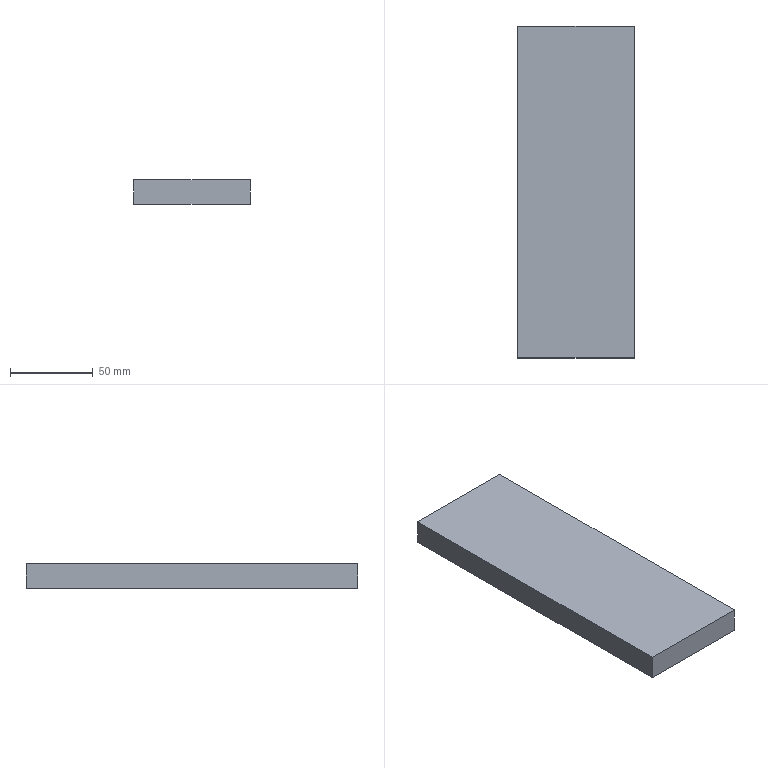Part | SolidWorks | features Extrusion 1 | 1 solid | 6 faces | box 70 x 200 x 15 mm | volume 210000 mm3 | plane 6
STEP:
#1=CARTESIAN_POINT('',(-35.,100.,-7.5));
#2=VERTEX_POINT('',#1);
#3=CARTESIAN_POINT('',(-35.,-100.,-7.5));
#4=VERTEX_POINT('',#3);
#5=CARTESIAN_POINT('',(-35.,-100.,-7.5));
#6=DIRECTION('',(0.,-1.,0.));
#7=VECTOR('',#6,1000.);
#8=LINE('',#5,#7);
#9=EDGE_CURVE('',#2,#4,#8,.T.);
#10=ORIENTED_EDGE('',*,*,#9,.T.);
#11=CARTESIAN_POINT('',(-35.,-100.,7.5));
#12=VERTEX_POINT('',#11);
#13=CARTESIAN_POINT('',(-35.,-100.,7.5));
#14=DIRECTION('',(0.,0.,-1.));
#15=VECTOR('',#14,1000.);
#16=LINE('',#13,#15);
#17=EDGE_CURVE('',#12,#4,#16,.T.);
#18=ORIENTED_EDGE('',*,*,#17,.F.);
#19=CARTESIAN_POINT('',(-35.,100.,7.5));
#20=VERTEX_POINT('',#19);
#21=CARTESIAN_POINT('',(-35.,-100.,7.5));
#22=DIRECTION('',(0.,-1.,0.));
#23=VECTOR('',#22,1000.);
#24=LINE('',#21,#23);
#25=EDGE_CURVE('',#20,#12,#24,.T.);
#26=ORIENTED_EDGE('',*,*,#25,.F.);
#27=CARTESIAN_POINT('',(-35.,100.,7.5));
#28=DIRECTION('',(0.,0.,-1.));
#29=VECTOR('',#28,1000.);
#30=LINE('',#27,#29);
#31=EDGE_CURVE('',#20,#2,#30,.T.);
#32=ORIENTED_EDGE('',*,*,#31,.T.);
#33=EDGE_LOOP('',(#10,#18,#26,#32));
#34=FACE_OUTER_BOUND('',#33,.T.);
#35=CARTESIAN_POINT('',(-35.,-100.,7.5));
#36=DIRECTION('',(1.,0.,0.));
#37=DIRECTION('',(0.,0.,-1.));
#38=AXIS2_PLACEMENT_3D('',#35,#36,#37);
#39=PLANE('',#38);
#40=ADVANCED_FACE('',(#34),#39,.F.);
#41=CARTESIAN_POINT('',(35.,-100.,-7.5));
#42=VERTEX_POINT('',#41);
#43=CARTESIAN_POINT('',(35.,-100.,-7.5));
#44=DIRECTION('',(1.,0.,0.));
#45=VECTOR('',#44,1000.);
#46=LINE('',#43,#45);
#47=EDGE_CURVE('',#4,#42,#46,.T.);
#48=ORIENTED_EDGE('',*,*,#47,.T.);
#49=CARTESIAN_POINT('',(35.,-100.,7.5));
#50=VERTEX_POINT('',#49);
#51=CARTESIAN_POINT('',(35.,-100.,7.5));
#52=DIRECTION('',(0.,0.,-1.));
#53=VECTOR('',#52,1000.);
#54=LINE('',#51,#53);
#55=EDGE_CURVE('',#50,#42,#54,.T.);
#56=ORIENTED_EDGE('',*,*,#55,.F.);
#57=CARTESIAN_POINT('',(35.,-100.,7.5));
#58=DIRECTION('',(1.,0.,0.));
#59=VECTOR('',#58,1000.);
#60=LINE('',#57,#59);
#61=EDGE_CURVE('',#12,#50,#60,.T.);
#62=ORIENTED_EDGE('',*,*,#61,.F.);
#63=ORIENTED_EDGE('',*,*,#17,.T.);
#64=EDGE_LOOP('',(#48,#56,#62,#63));
#65=FACE_OUTER_BOUND('',#64,.T.);
#66=CARTESIAN_POINT('',(35.,-100.,7.5));
#67=DIRECTION('',(0.,1.,0.));
#68=DIRECTION('',(0.,0.,1.));
#69=AXIS2_PLACEMENT_3D('',#66,#67,#68);
#70=PLANE('',#69);
#71=ADVANCED_FACE('',(#65),#70,.F.);
#72=CARTESIAN_POINT('',(35.,100.,-7.5));
#73=VERTEX_POINT('',#72);
#74=CARTESIAN_POINT('',(35.,-100.,-7.5));
#75=DIRECTION('',(0.,1.,0.));
#76=VECTOR('',#75,1000.);
#77=LINE('',#74,#76);
#78=EDGE_CURVE('',#42,#73,#77,.T.);
#79=ORIENTED_EDGE('',*,*,#78,.T.);
#80=CARTESIAN_POINT('',(35.,100.,7.5));
#81=VERTEX_POINT('',#80);
#82=CARTESIAN_POINT('',(35.,100.,7.5));
#83=DIRECTION('',(0.,0.,-1.));
#84=VECTOR('',#83,1000.);
#85=LINE('',#82,#84);
#86=EDGE_CURVE('',#81,#73,#85,.T.);
#87=ORIENTED_EDGE('',*,*,#86,.F.);
#88=CARTESIAN_POINT('',(35.,-100.,7.5));
#89=DIRECTION('',(0.,1.,0.));
#90=VECTOR('',#89,1000.);
#91=LINE('',#88,#90);
#92=EDGE_CURVE('',#50,#81,#91,.T.);
#93=ORIENTED_EDGE('',*,*,#92,.F.);
#94=ORIENTED_EDGE('',*,*,#55,.T.);
#95=EDGE_LOOP('',(#79,#87,#93,#94));
#96=FACE_OUTER_BOUND('',#95,.T.);
#97=CARTESIAN_POINT('',(35.,-100.,7.5));
#98=DIRECTION('',(-1.,0.,0.));
#99=DIRECTION('',(0.,0.,1.));
#100=AXIS2_PLACEMENT_3D('',#97,#98,#99);
#101=PLANE('',#100);
#102=ADVANCED_FACE('',(#96),#101,.F.);
#103=CARTESIAN_POINT('',(35.,100.,-7.5));
#104=DIRECTION('',(-1.,0.,0.));
#105=VECTOR('',#104,1000.);
#106=LINE('',#103,#105);
#107=EDGE_CURVE('',#73,#2,#106,.T.);
#108=ORIENTED_EDGE('',*,*,#107,.T.);
#109=ORIENTED_EDGE('',*,*,#31,.F.);
#110=CARTESIAN_POINT('',(35.,100.,7.5));
#111=DIRECTION('',(-1.,0.,0.));
#112=VECTOR('',#111,1000.);
#113=LINE('',#110,#112);
#114=EDGE_CURVE('',#81,#20,#113,.T.);
#115=ORIENTED_EDGE('',*,*,#114,.F.);
#116=ORIENTED_EDGE('',*,*,#86,.T.);
#117=EDGE_LOOP('',(#108,#109,#115,#116));
#118=FACE_OUTER_BOUND('',#117,.T.);
#119=CARTESIAN_POINT('',(35.,100.,7.5));
#120=DIRECTION('',(0.,-1.,0.));
#121=DIRECTION('',(1.,0.,0.));
#122=AXIS2_PLACEMENT_3D('',#119,#120,#121);
#123=PLANE('',#122);
#124=ADVANCED_FACE('',(#118),#123,.F.);
#125=ORIENTED_EDGE('',*,*,#25,.T.);
#126=ORIENTED_EDGE('',*,*,#61,.T.);
#127=ORIENTED_EDGE('',*,*,#92,.T.);
#128=ORIENTED_EDGE('',*,*,#114,.T.);
#129=EDGE_LOOP('',(#125,#126,#127,#128));
#130=FACE_OUTER_BOUND('',#129,.T.);
#131=CARTESIAN_POINT('',(0.,0.,7.5));
#132=DIRECTION('',(0.,0.,1.));
#133=DIRECTION('',(1.,0.,0.));
#134=AXIS2_PLACEMENT_3D('',#131,#132,#133);
#135=PLANE('',#134);
#136=ADVANCED_FACE('',(#130),#135,.T.);
#137=ORIENTED_EDGE('',*,*,#9,.F.);
#138=ORIENTED_EDGE('',*,*,#107,.F.);
#139=ORIENTED_EDGE('',*,*,#78,.F.);
#140=ORIENTED_EDGE('',*,*,#47,.F.);
#141=EDGE_LOOP('',(#137,#138,#139,#140));
#142=FACE_OUTER_BOUND('',#141,.T.);
#143=CARTESIAN_POINT('',(0.,0.,-7.5));
#144=DIRECTION('',(0.,0.,1.));
#145=DIRECTION('',(1.,0.,0.));
#146=AXIS2_PLACEMENT_3D('',#143,#144,#145);
#147=PLANE('',#146);
#148=ADVANCED_FACE('',(#142),#147,.F.);
#149=CLOSED_SHELL('',(#40,#71,#102,#124,#136,#148));
#150=MANIFOLD_SOLID_BREP('',#149);
#151=CARTESIAN_POINT('',(0.,0.,0.));
#152=DIRECTION('',(0.,0.,1.));
#153=DIRECTION('',(1.,0.,0.));
#154=AXIS2_PLACEMENT_3D('',#151,#152,#153);
#155=(LENGTH_UNIT()NAMED_UNIT(*)SI_UNIT(.MILLI.,.METRE.));
#156=UNCERTAINTY_MEASURE_WITH_UNIT(LENGTH_MEASURE(0.00001),#155,'','');
#157=(NAMED_UNIT(*)PLANE_ANGLE_UNIT()SI_UNIT($,.RADIAN.));
#158=(NAMED_UNIT(*)SI_UNIT($,.STERADIAN.)SOLID_ANGLE_UNIT());
#159=(GEOMETRIC_REPRESENTATION_CONTEXT(3)GLOBAL_UNCERTAINTY_ASSIGNED_CONTEXT((#156))GLOBAL_UNIT_ASSIGNED_CONTEXT((#155,#157,#158))REPRESENTATION_CONTEXT('',''));
#160=ADVANCED_BREP_SHAPE_REPRESENTATION('',(#150,#154),#159);